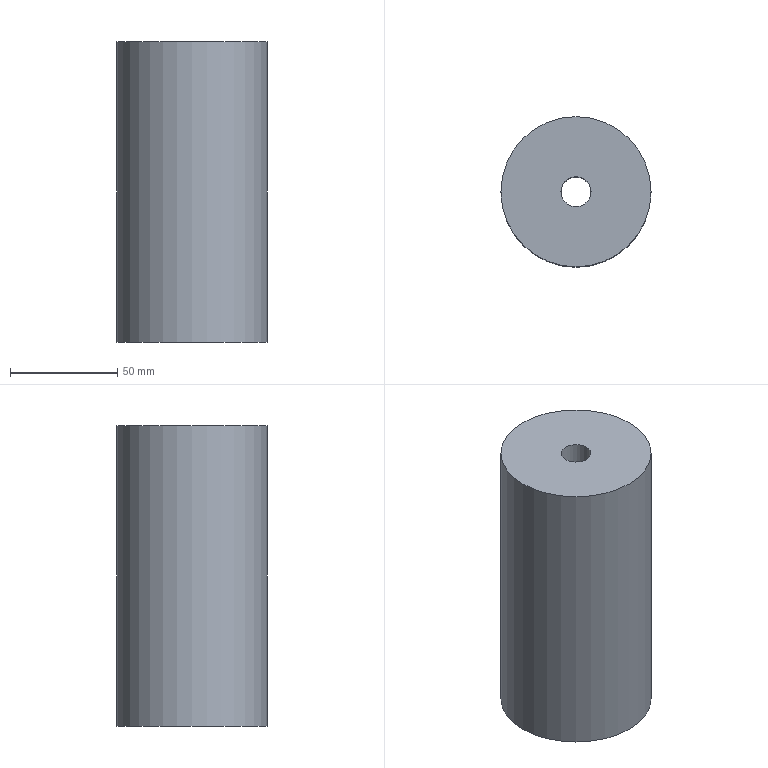Part | NX | features PHBTN70-140-110-Y_1 2 | 1 solid | 4 faces | box 70 x 70 x 140 mm | volume 517232 mm3 | cylinder 2 | plane 2 | commonest cylinder face diameters 14 x1 70 x1
STEP:
#1=CARTESIAN_POINT('',(3588.,607.5,-113.));
#2=VERTEX_POINT('',#1);
#3=CARTESIAN_POINT('',(3595.,607.5,-113.));
#4=DIRECTION('',(0.,0.,1.));
#5=DIRECTION('',(-1.,0.,0.));
#6=AXIS2_PLACEMENT_3D('',#3,#4,#5);
#7=CIRCLE('',#6,7.);
#8=EDGE_CURVE('',#2,#2,#7,.T.);
#9=ORIENTED_EDGE('',*,*,#8,.F.);
#10=EDGE_LOOP('',(#9));
#11=FACE_BOUND('',#10,.T.);
#12=CARTESIAN_POINT('',(3588.,607.5,27.));
#13=VERTEX_POINT('',#12);
#14=CARTESIAN_POINT('',(3595.,607.5,27.));
#15=DIRECTION('',(0.,0.,-1.));
#16=DIRECTION('',(-1.,0.,0.));
#17=AXIS2_PLACEMENT_3D('',#14,#15,#16);
#18=CIRCLE('',#17,7.);
#19=EDGE_CURVE('',#13,#13,#18,.T.);
#20=ORIENTED_EDGE('',*,*,#19,.F.);
#21=EDGE_LOOP('',(#20));
#22=FACE_BOUND('',#21,.T.);
#23=CARTESIAN_POINT('',(3595.,607.5,-43.));
#24=DIRECTION('',(0.,0.,1.));
#25=DIRECTION('',(-1.,0.,0.));
#26=AXIS2_PLACEMENT_3D('',#23,#24,#25);
#27=CYLINDRICAL_SURFACE('',#26,7.);
#28=ADVANCED_FACE('',(#11,#22),#27,.F.);
#29=CARTESIAN_POINT('',(3560.,607.5,-113.));
#30=VERTEX_POINT('',#29);
#31=CARTESIAN_POINT('',(3595.,607.5,-113.));
#32=DIRECTION('',(0.,0.,-1.));
#33=DIRECTION('',(-1.,0.,0.));
#34=AXIS2_PLACEMENT_3D('',#31,#32,#33);
#35=CIRCLE('',#34,35.);
#36=EDGE_CURVE('',#30,#30,#35,.T.);
#37=ORIENTED_EDGE('',*,*,#36,.F.);
#38=EDGE_LOOP('',(#37));
#39=FACE_BOUND('',#38,.T.);
#40=CARTESIAN_POINT('',(3560.,607.5,27.));
#41=VERTEX_POINT('',#40);
#42=CARTESIAN_POINT('',(3595.,607.5,27.));
#43=DIRECTION('',(0.,0.,1.));
#44=DIRECTION('',(-1.,0.,0.));
#45=AXIS2_PLACEMENT_3D('',#42,#43,#44);
#46=CIRCLE('',#45,35.);
#47=EDGE_CURVE('',#41,#41,#46,.T.);
#48=ORIENTED_EDGE('',*,*,#47,.F.);
#49=EDGE_LOOP('',(#48));
#50=FACE_BOUND('',#49,.T.);
#51=CARTESIAN_POINT('',(3595.,607.5,-43.));
#52=DIRECTION('',(0.,0.,1.));
#53=DIRECTION('',(-1.,0.,0.));
#54=AXIS2_PLACEMENT_3D('',#51,#52,#53);
#55=CYLINDRICAL_SURFACE('',#54,35.);
#56=ADVANCED_FACE('',(#39,#50),#55,.T.);
#57=ORIENTED_EDGE('',*,*,#8,.T.);
#58=EDGE_LOOP('',(#57));
#59=FACE_BOUND('',#58,.T.);
#60=ORIENTED_EDGE('',*,*,#36,.T.);
#61=EDGE_LOOP('',(#60));
#62=FACE_BOUND('',#61,.T.);
#63=CARTESIAN_POINT('',(3595.,607.5,-113.));
#64=DIRECTION('',(0.,0.,-1.));
#65=DIRECTION('',(1.,0.,0.));
#66=AXIS2_PLACEMENT_3D('',#63,#64,#65);
#67=PLANE('',#66);
#68=ADVANCED_FACE('',(#59,#62),#67,.T.);
#69=ORIENTED_EDGE('',*,*,#19,.T.);
#70=EDGE_LOOP('',(#69));
#71=FACE_BOUND('',#70,.T.);
#72=ORIENTED_EDGE('',*,*,#47,.T.);
#73=EDGE_LOOP('',(#72));
#74=FACE_BOUND('',#73,.T.);
#75=CARTESIAN_POINT('',(3595.,607.5,27.));
#76=DIRECTION('',(0.,0.,1.));
#77=DIRECTION('',(-1.,0.,0.));
#78=AXIS2_PLACEMENT_3D('',#75,#76,#77);
#79=PLANE('',#78);
#80=ADVANCED_FACE('',(#71,#74),#79,.T.);
#81=CLOSED_SHELL('',(#28,#56,#68,#80));
#82=MANIFOLD_SOLID_BREP('',#81);
#83=(LENGTH_UNIT()NAMED_UNIT(*)SI_UNIT(.MILLI.,.METRE.));
#84=UNCERTAINTY_MEASURE_WITH_UNIT(LENGTH_MEASURE(0.00001),#83,'','');
#85=(NAMED_UNIT(*)PLANE_ANGLE_UNIT()SI_UNIT($,.RADIAN.));
#86=(NAMED_UNIT(*)SI_UNIT($,.STERADIAN.)SOLID_ANGLE_UNIT());
#87=(GEOMETRIC_REPRESENTATION_CONTEXT(3)GLOBAL_UNCERTAINTY_ASSIGNED_CONTEXT((#84))GLOBAL_UNIT_ASSIGNED_CONTEXT((#83,#85,#86))REPRESENTATION_CONTEXT('',''));
#88=ADVANCED_BREP_SHAPE_REPRESENTATION('',(#82),#87);